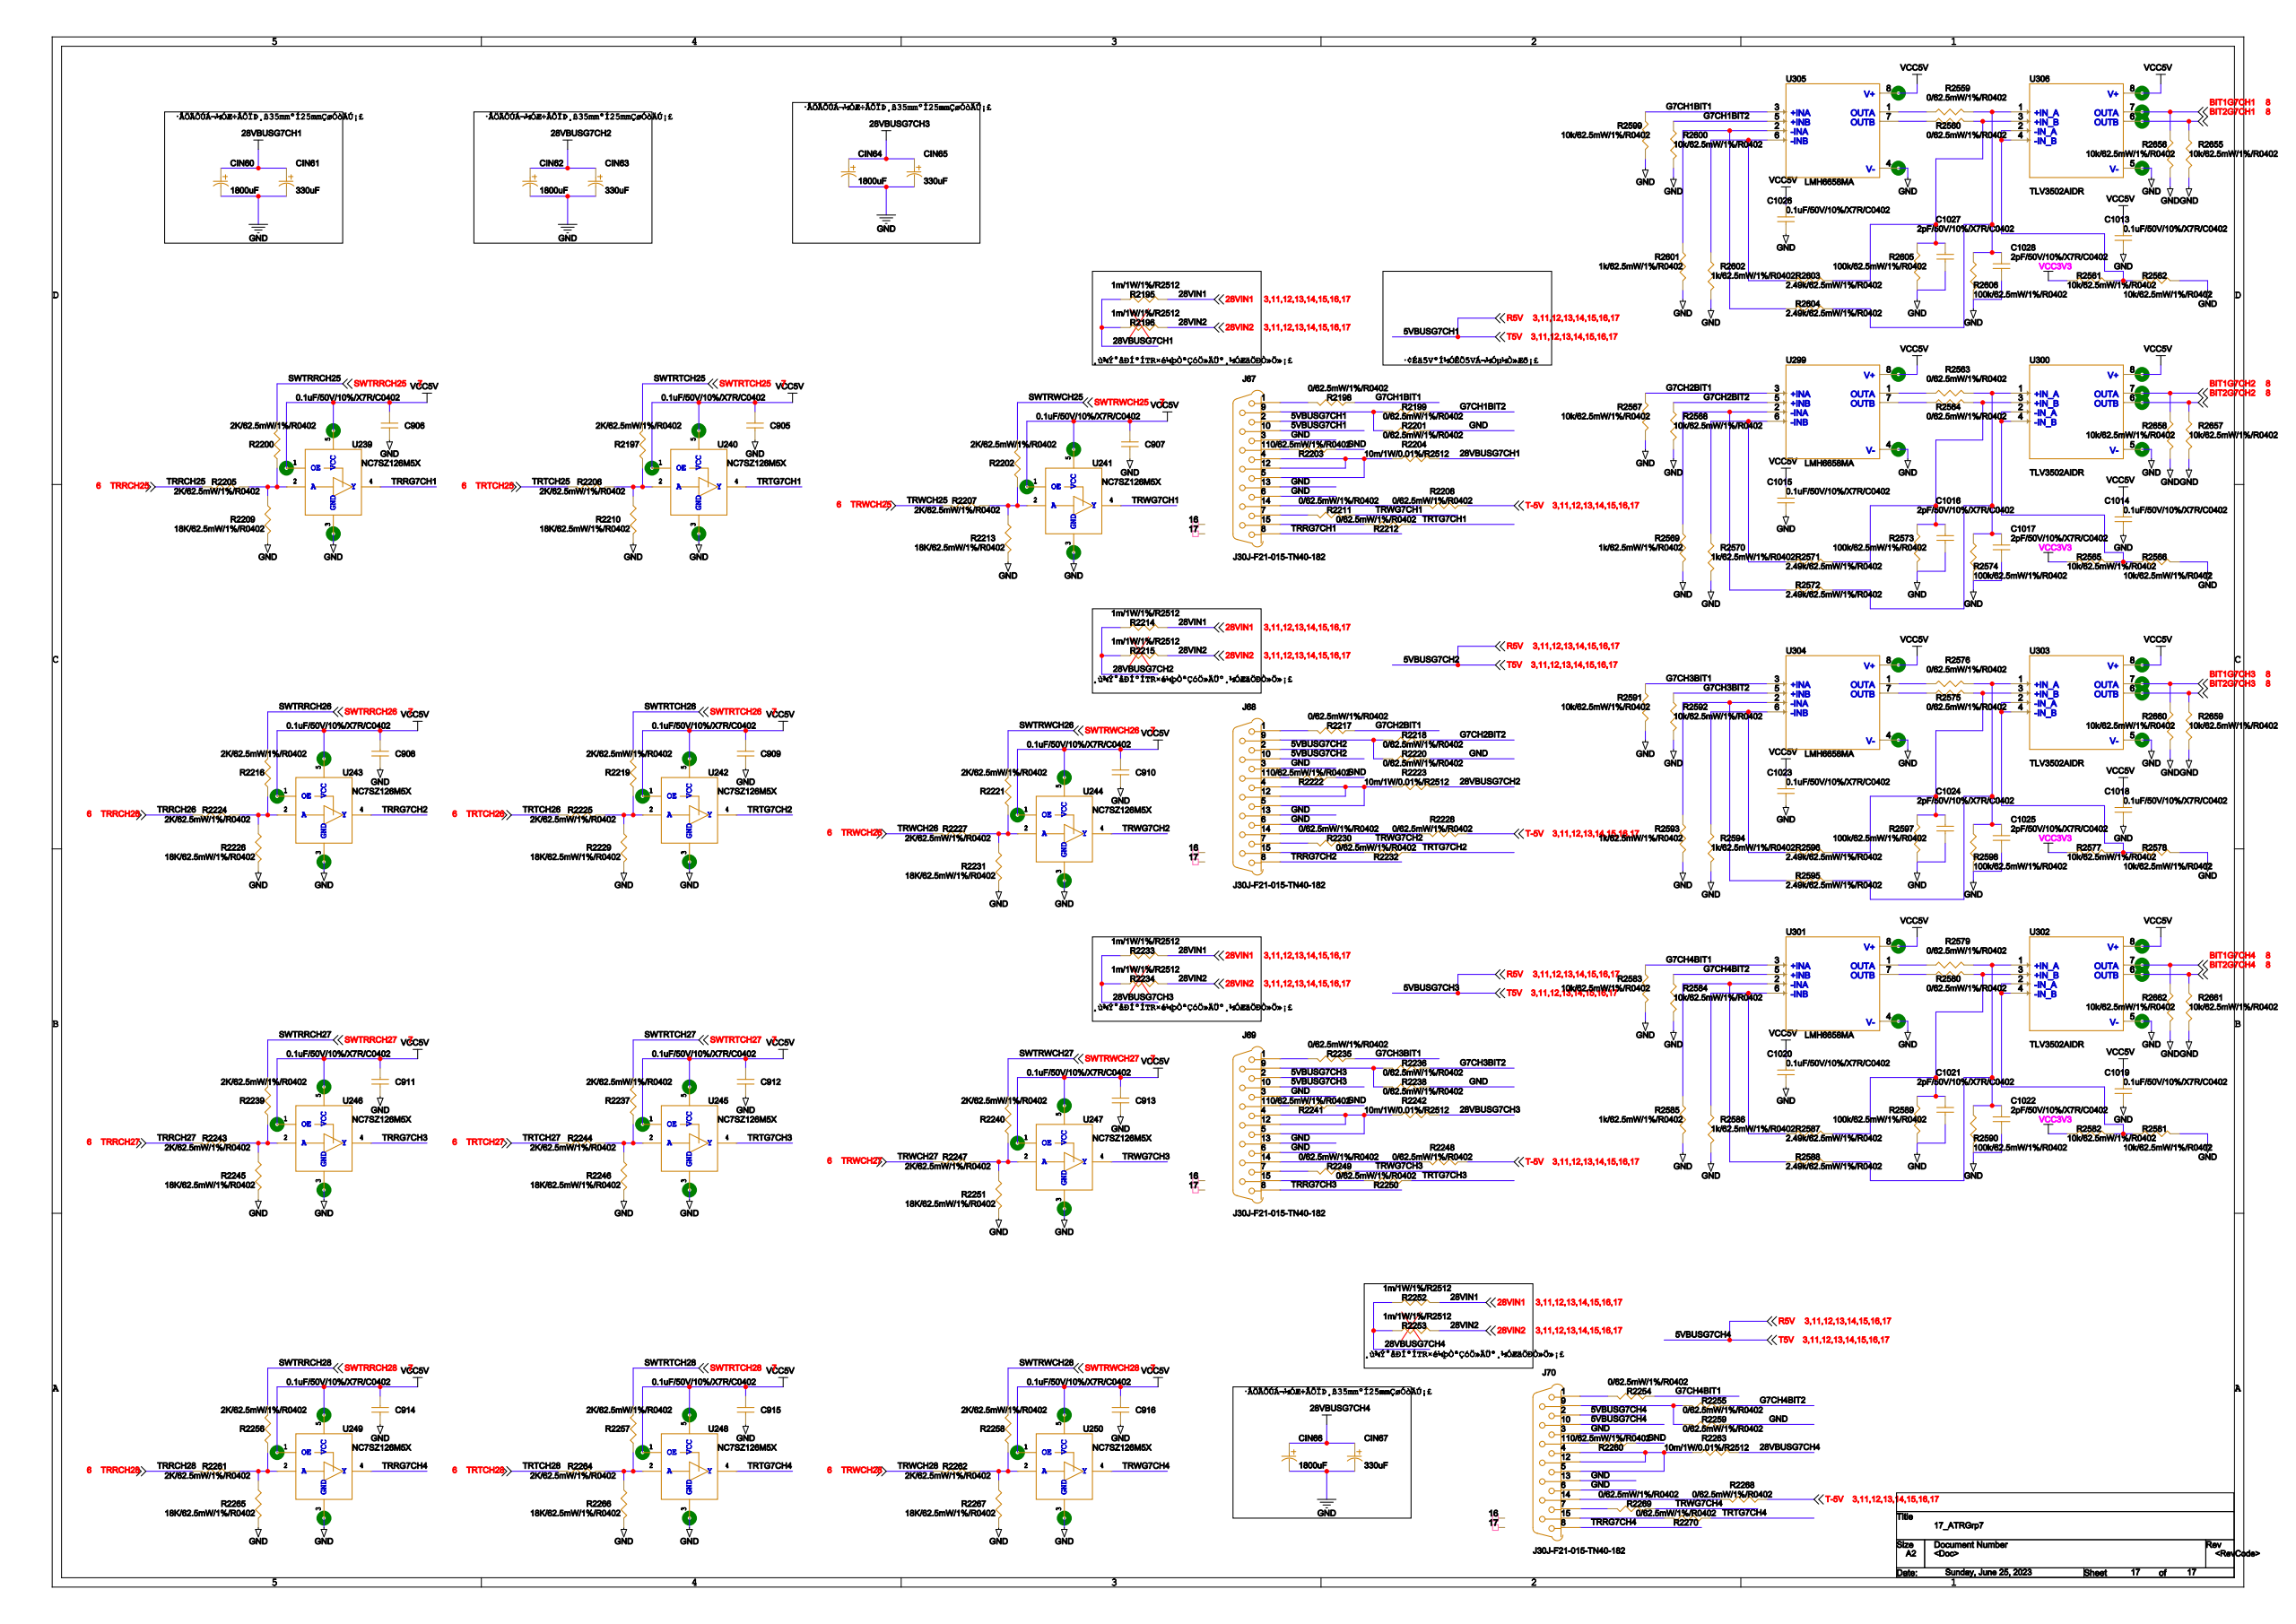Circuit board | Cadence Allegro | 1997 parts | 1536 nets | one sheet of the schematic
Parts on this sheet (reference | value | footprint):
C905 | 0.1uF/50V/10%/X7R/C0402 | 0402
C906 | 0.1uF/50V/10%/X7R/C0402 | 0402
C907 | 0.1uF/50V/10%/X7R/C0402 | 0402
C908 | 0.1uF/50V/10%/X7R/C0402 | 0402
C909 | 0.1uF/50V/10%/X7R/C0402 | 0402
C910 | 0.1uF/50V/10%/X7R/C0402 | 0402
C911 | 0.1uF/50V/10%/X7R/C0402 | 0402
C912 | 0.1uF/50V/10%/X7R/C0402 | 0402
C913 | 0.1uF/50V/10%/X7R/C0402 | 0402
C914 | 0.1uF/50V/10%/X7R/C0402 | 0402
C915 | 0.1uF/50V/10%/X7R/C0402 | 0402
C916 | 0.1uF/50V/10%/X7R/C0402 | 0402
C1013 | 0.1uF/50V/10%/X7R/C0402 | 0402
C1014 | 0.1uF/50V/10%/X7R/C0402 | 0402
C1016 | 2pF/50V/10%/X7R/C0402 | 0402
C1017 | 2pF/50V/10%/X7R/C0402 | 0402
C1018 | 0.1uF/50V/10%/X7R/C0402 | 0402
C1019 | 0.1uF/50V/10%/X7R/C0402 | 0402
C1021 | 2pF/50V/10%/X7R/C0402 | 0402
C1022 | 2pF/50V/10%/X7R/C0402 | 0402
C1024 | 2pF/50V/10%/X7R/C0402 | 0402
C1025 | 2pF/50V/10%/X7R/C0402 | 0402
C1027 | 2pF/50V/10%/X7R/C0402 | 0402
C1028 | 2pF/50V/10%/X7R/C0402 | 0402
CIN60 | ECF1HM182M27OTPO | AP-SMD_BD18-L27-W6_6-LS7_21
CIN61 | ECF1JM331G20OTPO | AP-SMD_BD10-L20-W6_6-LS7_21
CIN62 | ECF1HM182M27OTPO | AP-SMD_BD18-L27-W6_6-LS7_21
CIN63 | ECF1JM331G20OTPO | AP-SMD_BD10-L20-W6_6-LS7_21
CIN64 | ECF1HM182M27OTPO | AP-SMD_BD18-L27-W6_6-LS7_21
CIN65 | ECF1JM331G20OTPO | AP-SMD_BD10-L20-W6_6-LS7_21
CIN66 | ECF1HM182M27OTPO | AP-SMD_BD18-L27-W6_6-LS7_21
CIN67 | ECF1JM331G20OTPO | AP-SMD_BD10-L20-W6_6-LS7_21
J67 | J30J-F21-015-TN40-182 | J30J-F21-015-TN40-182
J68 | J30J-F21-015-TN40-182 | J30J-F21-015-TN40-182
J69 | J30J-F21-015-TN40-182 | J30J-F21-015-TN40-182
J70 | J30J-F21-015-TN40-182 | J30J-F21-015-TN40-182
R2195 | 1m/1W/1%/R2512 | 2512
R2196 | 1m/1W/1%/R2512 | 2512
R2197 | 2K/62.5mW/1%/R0402 | 0402
R2198 | 0/62.5mW/1%/R0402 | 0402
R2199 | 0/62.5mW/1%/R0402 | 0402
R2200 | 2K/62.5mW/1%/R0402 | 0402
R2201 | 0/62.5mW/1%/R0402 | 0402
R2202 | 2K/62.5mW/1%/R0402 | 0402
R2203 | 0/62.5mW/1%/R0402 | 0402
R2204 | 10m/1W/0.01%/R2512 | 2512
R2205 | 2K/62.5mW/1%/R0402 | 0402
R2206 | 2K/62.5mW/1%/R0402 | 0402
R2207 | 2K/62.5mW/1%/R0402 | 0402
R2208 | 0/62.5mW/1%/R0402 | 0402
R2209 | 18K/62.5mW/1%/R0402 | 0402
R2210 | 18K/62.5mW/1%/R0402 | 0402
R2211 | 0/62.5mW/1%/R0402 | 0402
R2212 | 0/62.5mW/1%/R0402 | 0402
R2213 | 18K/62.5mW/1%/R0402 | 0402
R2214 | 1m/1W/1%/R2512 | 2512
R2215 | 1m/1W/1%/R2512 | 2512
R2216 | 2K/62.5mW/1%/R0402 | 0402
R2217 | 0/62.5mW/1%/R0402 | 0402
R2218 | 0/62.5mW/1%/R0402 | 0402
R2219 | 2K/62.5mW/1%/R0402 | 0402
R2220 | 0/62.5mW/1%/R0402 | 0402
R2221 | 2K/62.5mW/1%/R0402 | 0402
R2222 | 0/62.5mW/1%/R0402 | 0402
R2223 | 10m/1W/0.01%/R2512 | 2512
R2224 | 2K/62.5mW/1%/R0402 | 0402
R2225 | 2K/62.5mW/1%/R0402 | 0402
R2226 | 18K/62.5mW/1%/R0402 | 0402
R2227 | 2K/62.5mW/1%/R0402 | 0402
R2228 | 0/62.5mW/1%/R0402 | 0402
R2229 | 18K/62.5mW/1%/R0402 | 0402
R2230 | 0/62.5mW/1%/R0402 | 0402
R2231 | 18K/62.5mW/1%/R0402 | 0402
R2232 | 0/62.5mW/1%/R0402 | 0402
R2233 | 1m/1W/1%/R2512 | 2512
R2234 | 1m/1W/1%/R2512 | 2512
R2235 | 0/62.5mW/1%/R0402 | 0402
R2236 | 0/62.5mW/1%/R0402 | 0402
R2237 | 2K/62.5mW/1%/R0402 | 0402
R2238 | 0/62.5mW/1%/R0402 | 0402
R2239 | 2K/62.5mW/1%/R0402 | 0402
R2240 | 2K/62.5mW/1%/R0402 | 0402
R2241 | 0/62.5mW/1%/R0402 | 0402
R2242 | 10m/1W/0.01%/R2512 | 2512
R2243 | 2K/62.5mW/1%/R0402 | 0402
R2244 | 2K/62.5mW/1%/R0402 | 0402
R2245 | 18K/62.5mW/1%/R0402 | 0402
R2246 | 18K/62.5mW/1%/R0402 | 0402
R2247 | 2K/62.5mW/1%/R0402 | 0402
R2248 | 0/62.5mW/1%/R0402 | 0402
R2249 | 0/62.5mW/1%/R0402 | 0402
R2250 | 0/62.5mW/1%/R0402 | 0402
R2251 | 18K/62.5mW/1%/R0402 | 0402
R2252 | 1m/1W/1%/R2512 | 2512
R2253 | 1m/1W/1%/R2512 | 2512
R2254 | 0/62.5mW/1%/R0402 | 0402
R2255 | 0/62.5mW/1%/R0402 | 0402
R2256 | 2K/62.5mW/1%/R0402 | 0402
R2257 | 2K/62.5mW/1%/R0402 | 0402
R2258 | 2K/62.5mW/1%/R0402 | 0402
R2259 | 0/62.5mW/1%/R0402 | 0402
R2260 | 0/62.5mW/1%/R0402 | 0402
R2261 | 2K/62.5mW/1%/R0402 | 0402
R2262 | 2K/62.5mW/1%/R0402 | 0402
R2263 | 10m/1W/0.01%/R2512 | 2512
R2264 | 2K/62.5mW/1%/R0402 | 0402
R2265 | 18K/62.5mW/1%/R0402 | 0402
R2266 | 18K/62.5mW/1%/R0402 | 0402
R2267 | 18K/62.5mW/1%/R0402 | 0402
R2268 | 0/62.5mW/1%/R0402 | 0402
R2269 | 0/62.5mW/1%/R0402 | 0402
R2270 | 0/62.5mW/1%/R0402 | 0402
R2559 | 0/62.5mW/1%/R0402 | 0402
R2560 | 0/62.5mW/1%/R0402 | 0402
R2561 | 10k/62.5mW/1%/R0402 | 0402
R2562 | 10k/62.5mW/1%/R0402 | 0402
R2563 | 0/62.5mW/1%/R0402 | 0402
R2564 | 0/62.5mW/1%/R0402 | 0402
R2565 | 10k/62.5mW/1%/R0402 | 0402
R2566 | 10k/62.5mW/1%/R0402 | 0402
R2567 | 10k/62.5mW/1%/R0402 | 0402
R2568 | 10k/62.5mW/1%/R0402 | 0402
R2569 | 1K/62.5mW/1%/R0402 | 0402
R2570 | 1K/62.5mW/1%/R0402 | 0402
R2572 | 2.49k/62.5mW/1%/R0402 | 0402
R2573 | 100k/62.5mW/1%/R0402 | 0402
R2574 | 100k/62.5mW/1%/R0402 | 0402
R2575 | 0/62.5mW/1%/R0402 | 0402
R2576 | 0/62.5mW/1%/R0402 | 0402
R2577 | 10k/62.5mW/1%/R0402 | 0402
R2578 | 10k/62.5mW/1%/R0402 | 0402
R2579 | 0/62.5mW/1%/R0402 | 0402
R2580 | 0/62.5mW/1%/R0402 | 0402
R2581 | 10k/62.5mW/1%/R0402 | 0402
R2582 | 10k/62.5mW/1%/R0402 | 0402
R2583 | 10k/62.5mW/1%/R0402 | 0402
R2584 | 10k/62.5mW/1%/R0402 | 0402
R2585 | 1K/62.5mW/1%/R0402 | 0402
R2586 | 1K/62.5mW/1%/R0402 | 0402
R2588 | 2.49k/62.5mW/1%/R0402 | 0402
R2589 | 100k/62.5mW/1%/R0402 | 0402
R2590 | 100k/62.5mW/1%/R0402 | 0402
R2591 | 10k/62.5mW/1%/R0402 | 0402
R2592 | 10k/62.5mW/1%/R0402 | 0402
R2593 | 1K/62.5mW/1%/R0402 | 0402
R2594 | 1K/62.5mW/1%/R0402 | 0402
R2595 | 2.49k/62.5mW/1%/R0402 | 0402
R2596 | 2.49k/62.5mW/1%/R0402 | 0402
R2597 | 100k/62.5mW/1%/R0402 | 0402
R2598 | 100k/62.5mW/1%/R0402 | 0402
R2599 | 10k/62.5mW/1%/R0402 | 0402
R2600 | 10k/62.5mW/1%/R0402 | 0402
R2601 | 1K/62.5mW/1%/R0402 | 0402
R2602 | 1K/62.5mW/1%/R0402 | 0402
R2604 | 2.49k/62.5mW/1%/R0402 | 0402
R2605 | 100k/62.5mW/1%/R0402 | 0402
R2606 | 100k/62.5mW/1%/R0402 | 0402
R2655 | 10k/62.5mW/1%/R0402 | 0402
R2656 | 10k/62.5mW/1%/R0402 | 0402
R2657 | 10k/62.5mW/1%/R0402 | 0402
R2658 | 10k/62.5mW/1%/R0402 | 0402
R2659 | 10k/62.5mW/1%/R0402 | 0402
R2660 | 10k/62.5mW/1%/R0402 | 0402
R2661 | 10k/62.5mW/1%/R0402 | 0402
R2662 | 10k/62.5mW/1%/R0402 | 0402
U239 | NC7SZ126M5X | SOT-23-5
U240 | NC7SZ126M5X | SOT-23-5
U241 | NC7SZ126M5X | SOT-23-5
U242 | NC7SZ126M5X | SOT-23-5
U243 | NC7SZ126M5X | SOT-23-5
U244 | NC7SZ126M5X | SOT-23-5
U245 | NC7SZ126M5X | SOT-23-5
U246 | NC7SZ126M5X | SOT-23-5
U247 | NC7SZ126M5X | SOT-23-5
U248 | NC7SZ126M5X | SOT-23-5
U249 | NC7SZ126M5X | SOT-23-5
U250 | NC7SZ126M5X | SOT-23-5
U299 | LMH6658MA | SOIC127P599X175-8N
U301 | LMH6658MA | SOIC127P599X175-8N
U303 | TLV3502AIDR | SOIC127P599X175-8N
U305 | LMH6658MA | SOIC127P599X175-8N
Nets of these parts (net: part-pin ...):
3.3V: R2561-1 R2565-1 R2577-1 R2582-1
AGND: C905-2 C906-2 C907-2 C908-2 C909-2 C910-2 C911-2 C912-2 C913-2 C914-2 C915-2 C916-2 C1013-2 C1014-2 C1016-2 C1017-2 C1018-2 C1019-2 C1021-2 C1022-2 C1024-2 C1025-2 C1027-2 C1028-2 CIN60-2 CIN61-2 CIN62-2 CIN63-2 CIN64-2 CIN65-2 CIN66-2 CIN67-2 J67-3 J67-6 J67-13 J68-3 J68-6 J68-13 J69-3 J69-6 J69-13 J70-3 J70-6 J70-13 R2201-1 R2203-1 R2209-1 R2210-1 R2213-1 R2220-1 R2222-1 R2226-1 R2229-1 R2231-1 R2238-1 R2241-1 R2245-1 R2246-1 R2251-1 R2259-1 R2260-1 R2265-1 R2266-1 R2267-1 R2562-2 R2566-2 R2567-2 R2568-2 R2569-2 R2570-2 R2573-2 R2574-2 R2578-2 R2581-2 R2583-2 R2584-2 R2585-2 R2586-2 R2589-2 R2590-2 R2591-2 R2592-2 R2593-2 R2594-2 R2597-2 R2598-2 R2599-2 R2600-2 R2601-2 R2602-2 R2605-2 R2606-2 R2655-2 R2656-2 R2657-2 R2658-2 R2659-2 R2660-2 R2661-2 R2662-2 U239-3 U240-3 U241-3 U242-3 U243-3 U244-3 U245-3 U246-3 U247-3 U248-3 U249-3 U250-3 U299-4 U301-4 U303-5 U305-4
VCC5V: C905-1 C906-1 C907-1 C908-1 C909-1 C910-1 C911-1 C912-1 C913-1 C914-1 C915-1 C916-1 C1013-1 C1014-1 C1018-1 C1019-1 U239-1 U239-5 U240-1 U240-5 U241-1 U241-5 U242-1 U242-5 U243-1 U243-5 U244-1 U244-5 U245-1 U245-5 U246-1 U246-5 U247-1 U247-5 U248-1 U248-5 U249-1 U249-5 U250-1 U250-5 U299-8 U301-8 U303-8 U305-8
N24412987: R2570-1 U299-6
N24412997: C1016-1 R2564-2 R2573-1
N24412975: R2569-1 R2572-1 U299-2
N24412995: C1017-1 R2563-2 R2572-2 R2574-1
N24413541: R2586-1 U301-6
N24413551: C1021-1 R2580-2 R2589-1
N24413529: R2585-1 R2588-1 U301-2
N24413549: C1022-1 R2579-2 R2588-2 R2590-1
N24413353: R2593-1 R2595-1
N24413369: C1025-1 R2576-2 R2595-2 R2598-1 U303-1
N24413357: R2594-1 R2596-1
N24413371: C1024-1 R2575-2 R2596-2 R2597-1 U303-3
N24412807: R2602-1 U305-6
N24412817: C1027-1 R2560-2 R2605-1
N24412803: R2601-1 R2604-1 U305-2
N24412815: C1028-1 R2559-2 R2604-2 R2606-1
G7CH2BIT1: R2217-1 R2567-1 U299-3
G7CH2BIT2: R2218-1 R2568-1 U299-5
N24412991: R2563-1 U299-1
N24412993: R2564-1 U299-7
G7CH4BIT1: R2254-1 R2583-1 U301-3
G7CH4BIT2: R2255-1 R2584-1 U301-5
N24413545: R2579-1 U301-1
N24413547: R2580-1 U301-7
G7CH3BIT1: R2235-1 R2591-1
G7CH3BIT2: R2236-1 R2592-1
N24413365: R2576-1
N24413367: R2575-1
G7CH1BIT1: R2198-1 R2599-1 U305-3
G7CH1BIT2: R2199-1 R2600-1 U305-5
N24412811: R2559-1 U305-1
N24412813: R2560-1 U305-7
N24413049: R2565-2 R2566-1
BIT1G7CH2: R2658-1
BIT2G7CH2: R2657-1
N24413603: R2581-1 R2582-2
BIT1G7CH4: R2662-1
BIT2G7CH4: R2661-1
N24413423: R2577-2 R2578-1 U303-2 U303-4
BIT1G7CH3: R2660-1 U303-7
BIT2G7CH3: R2659-1 U303-6
N24412869: R2561-2 R2562-1
BIT1G7CH1: R2656-1
BIT2G7CH1: R2655-1
R5V: J67-2 J67-10 J68-2 J68-10 J69-2 J69-10 J70-2 J70-10
N23736092: J67-1 R2198-2
N23736105: J67-11 R2203-2
N23736107: J67-4 J67-5 J67-12 R2204-1
N23736119: J67-14 R2208-2
N23736123: J67-15 R2212-2
N23736121: J67-7 R2211-2
TRRG7CH1: J67-8 U239-4
N23736094: J67-9 R2199-2 R2201-2
N23736651: J68-1 R2217-2
N23736664: J68-11 R2222-2
N23736666: J68-4 J68-5 J68-12 R2223-1
N23736678: J68-14 R2228-2
N23736682: J68-15 R2232-2
N23736680: J68-7 R2230-2
TRRG7CH2: J68-8 U243-4
N23736653: J68-9 R2218-2 R2220-2
N23737278: J69-1 R2235-2
N23737291: J69-11 R2241-2
N23737293: J69-4 J69-5 J69-12 R2242-1
N23737305: J69-14 R2248-2
N23737309: J69-15 R2250-2
N23737307: J69-7 R2249-2
TRRG7CH3: J69-8 U246-4
N23737280: J69-9 R2236-2 R2238-2
N23737910: J70-1 R2254-2
N23737923: J70-11 R2260-2
N23737925: J70-4 J70-5 J70-12 R2263-1
N23737937: J70-14 R2268-2
N23737941: J70-15 R2270-2
N23737939: J70-7 R2269-2
TRRG7CH4: J70-8 U249-4
N23737912: J70-9 R2255-2 R2259-2
28VIN1: R2195-2 R2214-2 R2233-2 R2252-2
T-5V: R2208-1 R2228-1 R2248-1 R2268-1
28VIN2: R2196-2 R2215-2 R2234-2 R2253-2
28VBUSG7CH1: CIN60-1 CIN61-1 R2195-1 R2196-1 R2204-2
28VBUSG7CH2: CIN62-1 CIN63-1 R2214-1 R2215-1 R2223-2
28VBUSG7CH3: CIN64-1 CIN65-1 R2233-1 R2234-1 R2242-2
28VBUSG7CH4: CIN66-1 CIN67-1 R2252-1 R2253-1 R2263-2
SWTRTCH25: R2197-1
N24020874: R2197-2 R2206-2 R2210-2 U240-2
SWTRRCH25: R2200-1
N24021854: R2200-2 R2205-2 R2209-2 U239-2
SWTRWCH25: R2202-1
N24021362: R2202-2 R2207-2 R2213-2 U241-2
TRRCH25: R2205-1
TRTCH25: R2206-1
TRWCH25: R2207-1
SWTRRCH26: R2216-1
N24021972: R2216-2 R2224-2 R2226-2 U243-2
SWTRTCH26: R2219-1
N24020992: R2219-2 R2225-2 R2229-2 U242-2
SWTRWCH26: R2221-1
N24021484: R2221-2 R2227-2 R2231-2 U244-2
TRRCH26: R2224-1
TRTCH26: R2225-1
TRWCH26: R2227-1
SWTRTCH27: R2237-1
N24021118: R2237-2 R2244-2 R2246-2 U245-2
SWTRRCH27: R2239-1
N24022098: R2239-2 R2243-2 R2245-2 U246-2
SWTRWCH27: R2240-1
N24021606: R2240-2 R2247-2 R2251-2 U247-2
TRRCH27: R2243-1
TRTCH27: R2244-1
TRWCH27: R2247-1
SWTRRCH28: R2256-1
N24022216: R2256-2 R2261-2 R2265-2 U249-2
SWTRTCH28: R2257-1
N24021240: R2257-2 R2264-2 R2266-2 U248-2
SWTRWCH28: R2258-1
N24021728: R2258-2 R2262-2 R2267-2 U250-2
TRRCH28: R2261-1
TRWCH28: R2262-1
TRTCH28: R2264-1
TRTG7CH1: R2212-1 U240-4
TRWG7CH1: R2211-1 U241-4
TRTG7CH2: R2232-1 U242-4
TRWG7CH2: R2230-1 U244-4
TRTG7CH3: R2250-1 U245-4
TRWG7CH3: R2249-1 U247-4
TRTG7CH4: R2270-1 U248-4
TRWG7CH4: R2269-1 U250-4